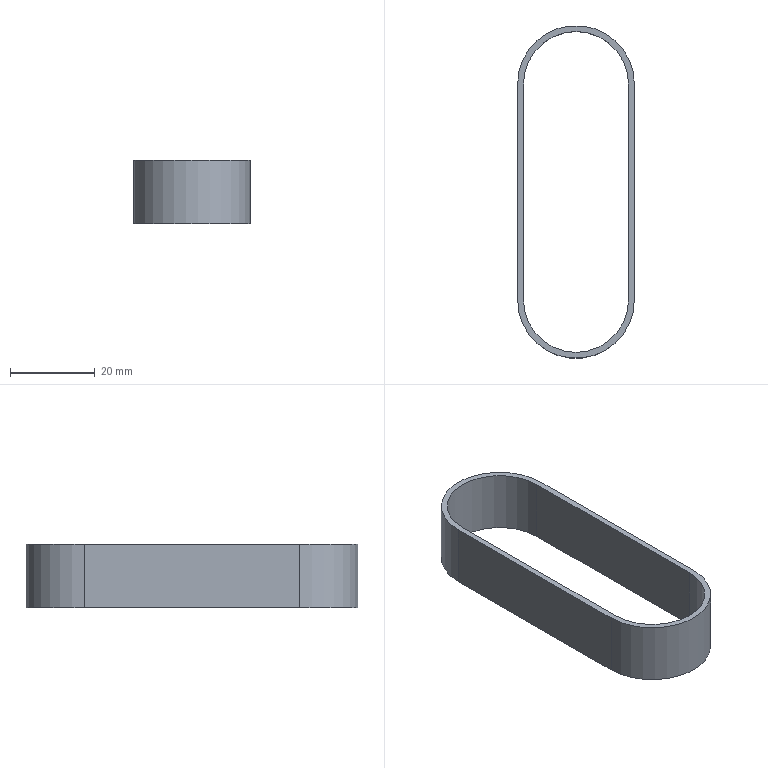Part | NX | features BREP 1 | 1 solid | 10 faces | box 27.59 x 78.59 x 15 mm | volume 3816 mm3 | plane 6 | cylinder 4 | commonest cylinder face diameters 24.83 x2 27.59 x2
STEP:
#1=CARTESIAN_POINT('',(-12.415,25.5,0.));
#2=VERTEX_POINT('',#1);
#3=CARTESIAN_POINT('',(-12.415,-25.5,0.));
#4=VERTEX_POINT('',#3);
#5=CARTESIAN_POINT('',(-12.415,-25.5,0.));
#6=DIRECTION('',(0.,-1.,0.));
#7=VECTOR('',#6,1000.);
#8=LINE('',#5,#7);
#9=EDGE_CURVE('',#2,#4,#8,.T.);
#10=ORIENTED_EDGE('',*,*,#9,.F.);
#11=CARTESIAN_POINT('',(-12.415,25.5,15.));
#12=VERTEX_POINT('',#11);
#13=CARTESIAN_POINT('',(-12.415,25.5,15.));
#14=DIRECTION('',(0.,0.,-1.));
#15=VECTOR('',#14,1000.);
#16=LINE('',#13,#15);
#17=EDGE_CURVE('',#12,#2,#16,.T.);
#18=ORIENTED_EDGE('',*,*,#17,.F.);
#19=CARTESIAN_POINT('',(-12.415,-25.5,15.));
#20=VERTEX_POINT('',#19);
#21=CARTESIAN_POINT('',(-12.415,-25.5,15.));
#22=DIRECTION('',(0.,-1.,0.));
#23=VECTOR('',#22,1000.);
#24=LINE('',#21,#23);
#25=EDGE_CURVE('',#12,#20,#24,.T.);
#26=ORIENTED_EDGE('',*,*,#25,.T.);
#27=CARTESIAN_POINT('',(-12.415,-25.5,15.));
#28=DIRECTION('',(0.,0.,-1.));
#29=VECTOR('',#28,1000.);
#30=LINE('',#27,#29);
#31=EDGE_CURVE('',#20,#4,#30,.T.);
#32=ORIENTED_EDGE('',*,*,#31,.T.);
#33=EDGE_LOOP('',(#10,#18,#26,#32));
#34=FACE_BOUND('',#33,.T.);
#35=CARTESIAN_POINT('',(-12.415,-25.5,15.));
#36=DIRECTION('',(1.,0.,0.));
#37=DIRECTION('',(0.,1.,0.));
#38=AXIS2_PLACEMENT_3D('',#35,#36,#37);
#39=PLANE('',#38);
#40=ADVANCED_FACE('',(#34),#39,.T.);
#41=CARTESIAN_POINT('',(12.415,25.5,0.));
#42=VERTEX_POINT('',#41);
#43=CARTESIAN_POINT('',(0.,25.5,0.));
#44=DIRECTION('',(0.,0.,1.));
#45=DIRECTION('',(1.,0.,0.));
#46=AXIS2_PLACEMENT_3D('',#43,#44,#45);
#47=CIRCLE('',#46,12.415);
#48=EDGE_CURVE('',#42,#2,#47,.T.);
#49=ORIENTED_EDGE('',*,*,#48,.F.);
#50=CARTESIAN_POINT('',(12.415,25.5,15.));
#51=VERTEX_POINT('',#50);
#52=CARTESIAN_POINT('',(12.415,25.5,15.));
#53=DIRECTION('',(0.,0.,-1.));
#54=VECTOR('',#53,1000.);
#55=LINE('',#52,#54);
#56=EDGE_CURVE('',#51,#42,#55,.T.);
#57=ORIENTED_EDGE('',*,*,#56,.F.);
#58=CARTESIAN_POINT('',(0.,25.5,15.));
#59=DIRECTION('',(0.,0.,1.));
#60=DIRECTION('',(1.,0.,0.));
#61=AXIS2_PLACEMENT_3D('',#58,#59,#60);
#62=CIRCLE('',#61,12.415);
#63=EDGE_CURVE('',#51,#12,#62,.T.);
#64=ORIENTED_EDGE('',*,*,#63,.T.);
#65=ORIENTED_EDGE('',*,*,#17,.T.);
#66=EDGE_LOOP('',(#49,#57,#64,#65));
#67=FACE_BOUND('',#66,.T.);
#68=CARTESIAN_POINT('',(0.,25.5,15.));
#69=DIRECTION('',(0.,0.,-1.));
#70=DIRECTION('',(-1.,0.,0.));
#71=AXIS2_PLACEMENT_3D('',#68,#69,#70);
#72=CYLINDRICAL_SURFACE('',#71,12.415);
#73=ADVANCED_FACE('',(#67),#72,.F.);
#74=CARTESIAN_POINT('',(12.415,-25.5,0.));
#75=VERTEX_POINT('',#74);
#76=CARTESIAN_POINT('',(12.415,-25.5,0.));
#77=DIRECTION('',(0.,1.,0.));
#78=VECTOR('',#77,1000.);
#79=LINE('',#76,#78);
#80=EDGE_CURVE('',#75,#42,#79,.T.);
#81=ORIENTED_EDGE('',*,*,#80,.F.);
#82=CARTESIAN_POINT('',(12.415,-25.5,15.));
#83=VERTEX_POINT('',#82);
#84=CARTESIAN_POINT('',(12.415,-25.5,15.));
#85=DIRECTION('',(0.,0.,-1.));
#86=VECTOR('',#85,1000.);
#87=LINE('',#84,#86);
#88=EDGE_CURVE('',#83,#75,#87,.T.);
#89=ORIENTED_EDGE('',*,*,#88,.F.);
#90=CARTESIAN_POINT('',(12.415,-25.5,15.));
#91=DIRECTION('',(0.,1.,0.));
#92=VECTOR('',#91,1000.);
#93=LINE('',#90,#92);
#94=EDGE_CURVE('',#83,#51,#93,.T.);
#95=ORIENTED_EDGE('',*,*,#94,.T.);
#96=ORIENTED_EDGE('',*,*,#56,.T.);
#97=EDGE_LOOP('',(#81,#89,#95,#96));
#98=FACE_BOUND('',#97,.T.);
#99=CARTESIAN_POINT('',(12.415,-25.5,15.));
#100=DIRECTION('',(-1.,0.,0.));
#101=DIRECTION('',(0.,-1.,0.));
#102=AXIS2_PLACEMENT_3D('',#99,#100,#101);
#103=PLANE('',#102);
#104=ADVANCED_FACE('',(#98),#103,.T.);
#105=CARTESIAN_POINT('',(0.,-25.5,0.));
#106=DIRECTION('',(0.,0.,1.));
#107=DIRECTION('',(1.,0.,0.));
#108=AXIS2_PLACEMENT_3D('',#105,#106,#107);
#109=CIRCLE('',#108,12.415);
#110=EDGE_CURVE('',#4,#75,#109,.T.);
#111=ORIENTED_EDGE('',*,*,#110,.F.);
#112=ORIENTED_EDGE('',*,*,#31,.F.);
#113=CARTESIAN_POINT('',(0.,-25.5,15.));
#114=DIRECTION('',(0.,0.,1.));
#115=DIRECTION('',(1.,0.,0.));
#116=AXIS2_PLACEMENT_3D('',#113,#114,#115);
#117=CIRCLE('',#116,12.415);
#118=EDGE_CURVE('',#20,#83,#117,.T.);
#119=ORIENTED_EDGE('',*,*,#118,.T.);
#120=ORIENTED_EDGE('',*,*,#88,.T.);
#121=EDGE_LOOP('',(#111,#112,#119,#120));
#122=FACE_BOUND('',#121,.T.);
#123=CARTESIAN_POINT('',(0.,-25.5,15.));
#124=DIRECTION('',(0.,0.,-1.));
#125=DIRECTION('',(-1.,0.,0.));
#126=AXIS2_PLACEMENT_3D('',#123,#124,#125);
#127=CYLINDRICAL_SURFACE('',#126,12.415);
#128=ADVANCED_FACE('',(#122),#127,.F.);
#129=CARTESIAN_POINT('',(-13.795,25.5,0.));
#130=VERTEX_POINT('',#129);
#131=CARTESIAN_POINT('',(-13.795,-25.5,0.));
#132=VERTEX_POINT('',#131);
#133=CARTESIAN_POINT('',(-13.795,-25.5,0.));
#134=DIRECTION('',(0.,-1.,0.));
#135=VECTOR('',#134,1000.);
#136=LINE('',#133,#135);
#137=EDGE_CURVE('',#130,#132,#136,.T.);
#138=ORIENTED_EDGE('',*,*,#137,.T.);
#139=CARTESIAN_POINT('',(-13.795,-25.5,15.));
#140=VERTEX_POINT('',#139);
#141=CARTESIAN_POINT('',(-13.795,-25.5,15.));
#142=DIRECTION('',(0.,0.,-1.));
#143=VECTOR('',#142,1000.);
#144=LINE('',#141,#143);
#145=EDGE_CURVE('',#140,#132,#144,.T.);
#146=ORIENTED_EDGE('',*,*,#145,.F.);
#147=CARTESIAN_POINT('',(-13.795,25.5,15.));
#148=VERTEX_POINT('',#147);
#149=CARTESIAN_POINT('',(-13.795,-25.5,15.));
#150=DIRECTION('',(0.,-1.,0.));
#151=VECTOR('',#150,1000.);
#152=LINE('',#149,#151);
#153=EDGE_CURVE('',#148,#140,#152,.T.);
#154=ORIENTED_EDGE('',*,*,#153,.F.);
#155=CARTESIAN_POINT('',(-13.795,25.5,15.));
#156=DIRECTION('',(0.,0.,-1.));
#157=VECTOR('',#156,1000.);
#158=LINE('',#155,#157);
#159=EDGE_CURVE('',#148,#130,#158,.T.);
#160=ORIENTED_EDGE('',*,*,#159,.T.);
#161=EDGE_LOOP('',(#138,#146,#154,#160));
#162=FACE_BOUND('',#161,.T.);
#163=CARTESIAN_POINT('',(-13.795,-25.5,15.));
#164=DIRECTION('',(1.,0.,0.));
#165=DIRECTION('',(0.,1.,0.));
#166=AXIS2_PLACEMENT_3D('',#163,#164,#165);
#167=PLANE('',#166);
#168=ADVANCED_FACE('',(#162),#167,.F.);
#169=CARTESIAN_POINT('',(13.795,25.5,0.));
#170=VERTEX_POINT('',#169);
#171=CARTESIAN_POINT('',(0.,25.5,0.));
#172=DIRECTION('',(0.,0.,1.));
#173=DIRECTION('',(1.,0.,0.));
#174=AXIS2_PLACEMENT_3D('',#171,#172,#173);
#175=CIRCLE('',#174,13.795);
#176=EDGE_CURVE('',#170,#130,#175,.T.);
#177=ORIENTED_EDGE('',*,*,#176,.T.);
#178=ORIENTED_EDGE('',*,*,#159,.F.);
#179=CARTESIAN_POINT('',(13.795,25.5,15.));
#180=VERTEX_POINT('',#179);
#181=CARTESIAN_POINT('',(0.,25.5,15.));
#182=DIRECTION('',(0.,0.,1.));
#183=DIRECTION('',(1.,0.,0.));
#184=AXIS2_PLACEMENT_3D('',#181,#182,#183);
#185=CIRCLE('',#184,13.795);
#186=EDGE_CURVE('',#180,#148,#185,.T.);
#187=ORIENTED_EDGE('',*,*,#186,.F.);
#188=CARTESIAN_POINT('',(13.795,25.5,15.));
#189=DIRECTION('',(0.,0.,-1.));
#190=VECTOR('',#189,1000.);
#191=LINE('',#188,#190);
#192=EDGE_CURVE('',#180,#170,#191,.T.);
#193=ORIENTED_EDGE('',*,*,#192,.T.);
#194=EDGE_LOOP('',(#177,#178,#187,#193));
#195=FACE_BOUND('',#194,.T.);
#196=CARTESIAN_POINT('',(0.,25.5,15.));
#197=DIRECTION('',(0.,0.,-1.));
#198=DIRECTION('',(-1.,0.,0.));
#199=AXIS2_PLACEMENT_3D('',#196,#197,#198);
#200=CYLINDRICAL_SURFACE('',#199,13.795);
#201=ADVANCED_FACE('',(#195),#200,.T.);
#202=CARTESIAN_POINT('',(13.795,-25.5,0.));
#203=VERTEX_POINT('',#202);
#204=CARTESIAN_POINT('',(13.795,-25.5,0.));
#205=DIRECTION('',(0.,1.,0.));
#206=VECTOR('',#205,1000.);
#207=LINE('',#204,#206);
#208=EDGE_CURVE('',#203,#170,#207,.T.);
#209=ORIENTED_EDGE('',*,*,#208,.T.);
#210=ORIENTED_EDGE('',*,*,#192,.F.);
#211=CARTESIAN_POINT('',(13.795,-25.5,15.));
#212=VERTEX_POINT('',#211);
#213=CARTESIAN_POINT('',(13.795,-25.5,15.));
#214=DIRECTION('',(0.,1.,0.));
#215=VECTOR('',#214,1000.);
#216=LINE('',#213,#215);
#217=EDGE_CURVE('',#212,#180,#216,.T.);
#218=ORIENTED_EDGE('',*,*,#217,.F.);
#219=CARTESIAN_POINT('',(13.795,-25.5,15.));
#220=DIRECTION('',(0.,0.,-1.));
#221=VECTOR('',#220,1000.);
#222=LINE('',#219,#221);
#223=EDGE_CURVE('',#212,#203,#222,.T.);
#224=ORIENTED_EDGE('',*,*,#223,.T.);
#225=EDGE_LOOP('',(#209,#210,#218,#224));
#226=FACE_BOUND('',#225,.T.);
#227=CARTESIAN_POINT('',(13.795,-25.5,15.));
#228=DIRECTION('',(-1.,0.,0.));
#229=DIRECTION('',(0.,-1.,0.));
#230=AXIS2_PLACEMENT_3D('',#227,#228,#229);
#231=PLANE('',#230);
#232=ADVANCED_FACE('',(#226),#231,.F.);
#233=CARTESIAN_POINT('',(0.,-25.5,0.));
#234=DIRECTION('',(0.,0.,1.));
#235=DIRECTION('',(1.,0.,0.));
#236=AXIS2_PLACEMENT_3D('',#233,#234,#235);
#237=CIRCLE('',#236,13.795);
#238=EDGE_CURVE('',#132,#203,#237,.T.);
#239=ORIENTED_EDGE('',*,*,#238,.T.);
#240=ORIENTED_EDGE('',*,*,#223,.F.);
#241=CARTESIAN_POINT('',(0.,-25.5,15.));
#242=DIRECTION('',(0.,0.,1.));
#243=DIRECTION('',(1.,0.,0.));
#244=AXIS2_PLACEMENT_3D('',#241,#242,#243);
#245=CIRCLE('',#244,13.795);
#246=EDGE_CURVE('',#140,#212,#245,.T.);
#247=ORIENTED_EDGE('',*,*,#246,.F.);
#248=ORIENTED_EDGE('',*,*,#145,.T.);
#249=EDGE_LOOP('',(#239,#240,#247,#248));
#250=FACE_BOUND('',#249,.T.);
#251=CARTESIAN_POINT('',(0.,-25.5,15.));
#252=DIRECTION('',(0.,0.,-1.));
#253=DIRECTION('',(-1.,0.,0.));
#254=AXIS2_PLACEMENT_3D('',#251,#252,#253);
#255=CYLINDRICAL_SURFACE('',#254,13.795);
#256=ADVANCED_FACE('',(#250),#255,.T.);
#257=ORIENTED_EDGE('',*,*,#110,.T.);
#258=ORIENTED_EDGE('',*,*,#80,.T.);
#259=ORIENTED_EDGE('',*,*,#48,.T.);
#260=ORIENTED_EDGE('',*,*,#9,.T.);
#261=EDGE_LOOP('',(#257,#258,#259,#260));
#262=FACE_BOUND('',#261,.T.);
#263=ORIENTED_EDGE('',*,*,#238,.F.);
#264=ORIENTED_EDGE('',*,*,#137,.F.);
#265=ORIENTED_EDGE('',*,*,#176,.F.);
#266=ORIENTED_EDGE('',*,*,#208,.F.);
#267=EDGE_LOOP('',(#263,#264,#265,#266));
#268=FACE_BOUND('',#267,.T.);
#269=CARTESIAN_POINT('',(0.,-25.5,0.));
#270=DIRECTION('',(0.,0.,1.));
#271=DIRECTION('',(1.,0.,0.));
#272=AXIS2_PLACEMENT_3D('',#269,#270,#271);
#273=PLANE('',#272);
#274=ADVANCED_FACE('',(#262,#268),#273,.F.);
#275=ORIENTED_EDGE('',*,*,#94,.F.);
#276=ORIENTED_EDGE('',*,*,#118,.F.);
#277=ORIENTED_EDGE('',*,*,#25,.F.);
#278=ORIENTED_EDGE('',*,*,#63,.F.);
#279=EDGE_LOOP('',(#275,#276,#277,#278));
#280=FACE_BOUND('',#279,.T.);
#281=ORIENTED_EDGE('',*,*,#246,.T.);
#282=ORIENTED_EDGE('',*,*,#217,.T.);
#283=ORIENTED_EDGE('',*,*,#186,.T.);
#284=ORIENTED_EDGE('',*,*,#153,.T.);
#285=EDGE_LOOP('',(#281,#282,#283,#284));
#286=FACE_BOUND('',#285,.T.);
#287=CARTESIAN_POINT('',(0.,-25.5,15.));
#288=DIRECTION('',(0.,0.,1.));
#289=DIRECTION('',(1.,0.,0.));
#290=AXIS2_PLACEMENT_3D('',#287,#288,#289);
#291=PLANE('',#290);
#292=ADVANCED_FACE('',(#280,#286),#291,.T.);
#293=CLOSED_SHELL('',(#40,#73,#104,#128,#168,#201,#232,#256,#274,#292));
#294=MANIFOLD_SOLID_BREP('',#293);
#295=(LENGTH_UNIT()NAMED_UNIT(*)SI_UNIT(.MILLI.,.METRE.));
#296=UNCERTAINTY_MEASURE_WITH_UNIT(LENGTH_MEASURE(0.00001),#295,'','');
#297=(NAMED_UNIT(*)PLANE_ANGLE_UNIT()SI_UNIT($,.RADIAN.));
#298=(NAMED_UNIT(*)SI_UNIT($,.STERADIAN.)SOLID_ANGLE_UNIT());
#299=(GEOMETRIC_REPRESENTATION_CONTEXT(3)GLOBAL_UNCERTAINTY_ASSIGNED_CONTEXT((#296))GLOBAL_UNIT_ASSIGNED_CONTEXT((#295,#297,#298))REPRESENTATION_CONTEXT('',''));
#300=ADVANCED_BREP_SHAPE_REPRESENTATION('',(#294),#299);